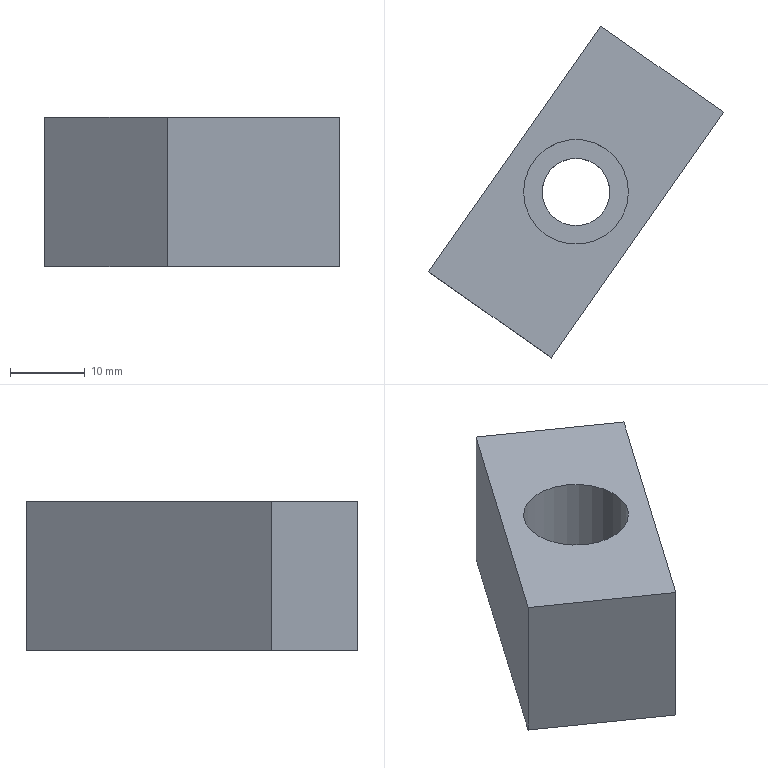Part | NX | features solid 2 | 1 solid | 9 faces | box 39.326 x 44.238 x 20 mm | volume 13824 mm3 | plane 7 | cylinder 2 | commonest cylinder face diameters 9 x1 14 x1
STEP:
#1=CARTESIAN_POINT('',(61.729,209.988,-474.059));
#2=VERTEX_POINT('',#1);
#3=CARTESIAN_POINT('',(66.229,209.988,-474.059));
#4=DIRECTION('',(0.,0.,-1.));
#5=DIRECTION('',(-1.,0.,0.));
#6=AXIS2_PLACEMENT_3D('',#3,#4,#5);
#7=CIRCLE('',#6,4.5);
#8=EDGE_CURVE('',#2,#2,#7,.T.);
#9=ORIENTED_EDGE('',*,*,#8,.F.);
#10=EDGE_LOOP('',(#9));
#11=FACE_BOUND('',#10,.T.);
#12=CARTESIAN_POINT('',(46.566,199.341,-474.059));
#13=VERTEX_POINT('',#12);
#14=CARTESIAN_POINT('',(62.949,187.87,-474.059));
#15=VERTEX_POINT('',#14);
#16=CARTESIAN_POINT('',(79.332,176.398,-474.059));
#17=DIRECTION('',(0.8192,-0.5736,0.));
#18=VECTOR('',#17,1000.);
#19=LINE('',#16,#18);
#20=EDGE_CURVE('',#13,#15,#19,.T.);
#21=ORIENTED_EDGE('',*,*,#20,.F.);
#22=CARTESIAN_POINT('',(69.509,232.107,-474.059));
#23=VERTEX_POINT('',#22);
#24=CARTESIAN_POINT('',(35.381,183.368,-474.059));
#25=DIRECTION('',(0.5736,0.8192,0.));
#26=VECTOR('',#25,1000.);
#27=LINE('',#24,#26);
#28=EDGE_CURVE('',#13,#23,#27,.T.);
#29=ORIENTED_EDGE('',*,*,#28,.T.);
#30=CARTESIAN_POINT('',(85.892,220.636,-474.059));
#31=VERTEX_POINT('',#30);
#32=CARTESIAN_POINT('',(69.509,232.107,-474.059));
#33=DIRECTION('',(0.8192,-0.5736,0.));
#34=VECTOR('',#33,1000.);
#35=LINE('',#32,#34);
#36=EDGE_CURVE('',#23,#31,#35,.T.);
#37=ORIENTED_EDGE('',*,*,#36,.T.);
#38=CARTESIAN_POINT('',(51.765,171.896,-474.059));
#39=DIRECTION('',(0.5736,0.8192,0.));
#40=VECTOR('',#39,1000.);
#41=LINE('',#38,#40);
#42=EDGE_CURVE('',#15,#31,#41,.T.);
#43=ORIENTED_EDGE('',*,*,#42,.F.);
#44=EDGE_LOOP('',(#21,#29,#37,#43));
#45=FACE_BOUND('',#44,.T.);
#46=CARTESIAN_POINT('',(35.381,183.368,-474.059));
#47=DIRECTION('',(0.,0.,-1.));
#48=DIRECTION('',(0.5736,0.8192,0.));
#49=AXIS2_PLACEMENT_3D('',#46,#47,#48);
#50=PLANE('',#49);
#51=ADVANCED_FACE('',(#11,#45),#50,.T.);
#52=ORIENTED_EDGE('',*,*,#36,.F.);
#53=CARTESIAN_POINT('',(69.509,232.107,-454.059));
#54=VERTEX_POINT('',#53);
#55=CARTESIAN_POINT('',(69.509,232.107,-474.059));
#56=DIRECTION('',(0.,0.,1.));
#57=VECTOR('',#56,1000.);
#58=LINE('',#55,#57);
#59=EDGE_CURVE('',#23,#54,#58,.T.);
#60=ORIENTED_EDGE('',*,*,#59,.T.);
#61=CARTESIAN_POINT('',(85.892,220.636,-454.059));
#62=VERTEX_POINT('',#61);
#63=CARTESIAN_POINT('',(69.509,232.107,-454.059));
#64=DIRECTION('',(-0.8192,0.5736,0.));
#65=VECTOR('',#64,1000.);
#66=LINE('',#63,#65);
#67=EDGE_CURVE('',#54,#62,#66,.F.);
#68=ORIENTED_EDGE('',*,*,#67,.T.);
#69=CARTESIAN_POINT('',(85.892,220.636,-474.059));
#70=DIRECTION('',(0.,0.,1.));
#71=VECTOR('',#70,1000.);
#72=LINE('',#69,#71);
#73=EDGE_CURVE('',#31,#62,#72,.T.);
#74=ORIENTED_EDGE('',*,*,#73,.F.);
#75=EDGE_LOOP('',(#52,#60,#68,#74));
#76=FACE_BOUND('',#75,.T.);
#77=CARTESIAN_POINT('',(69.509,232.107,-394.059));
#78=DIRECTION('',(0.5736,0.8192,0.));
#79=DIRECTION('',(0.,0.,1.));
#80=AXIS2_PLACEMENT_3D('',#77,#78,#79);
#81=PLANE('',#80);
#82=ADVANCED_FACE('',(#76),#81,.T.);
#83=CARTESIAN_POINT('',(59.229,209.988,-454.059));
#84=VERTEX_POINT('',#83);
#85=CARTESIAN_POINT('',(66.229,209.988,-454.059));
#86=DIRECTION('',(0.,0.,-1.));
#87=DIRECTION('',(-1.,0.,0.));
#88=AXIS2_PLACEMENT_3D('',#85,#86,#87);
#89=CIRCLE('',#88,7.);
#90=EDGE_CURVE('',#84,#84,#89,.T.);
#91=ORIENTED_EDGE('',*,*,#90,.T.);
#92=EDGE_LOOP('',(#91));
#93=FACE_BOUND('',#92,.T.);
#94=ORIENTED_EDGE('',*,*,#67,.F.);
#95=CARTESIAN_POINT('',(46.566,199.341,-454.059));
#96=VERTEX_POINT('',#95);
#97=CARTESIAN_POINT('',(35.381,183.368,-454.059));
#98=DIRECTION('',(0.5736,0.8192,0.));
#99=VECTOR('',#98,1000.);
#100=LINE('',#97,#99);
#101=EDGE_CURVE('',#96,#54,#100,.T.);
#102=ORIENTED_EDGE('',*,*,#101,.F.);
#103=CARTESIAN_POINT('',(62.949,187.87,-454.059));
#104=VERTEX_POINT('',#103);
#105=CARTESIAN_POINT('',(46.566,199.341,-454.059));
#106=DIRECTION('',(-0.8192,0.5736,0.));
#107=VECTOR('',#106,1000.);
#108=LINE('',#105,#107);
#109=EDGE_CURVE('',#96,#104,#108,.F.);
#110=ORIENTED_EDGE('',*,*,#109,.T.);
#111=CARTESIAN_POINT('',(51.765,171.896,-454.059));
#112=DIRECTION('',(0.5736,0.8192,0.));
#113=VECTOR('',#112,1000.);
#114=LINE('',#111,#113);
#115=EDGE_CURVE('',#104,#62,#114,.T.);
#116=ORIENTED_EDGE('',*,*,#115,.T.);
#117=EDGE_LOOP('',(#94,#102,#110,#116));
#118=FACE_BOUND('',#117,.T.);
#119=CARTESIAN_POINT('',(35.381,183.368,-454.059));
#120=DIRECTION('',(0.,0.,-1.));
#121=DIRECTION('',(0.5736,0.8192,0.));
#122=AXIS2_PLACEMENT_3D('',#119,#120,#121);
#123=PLANE('',#122);
#124=ADVANCED_FACE('',(#93,#118),#123,.F.);
#125=ORIENTED_EDGE('',*,*,#115,.F.);
#126=CARTESIAN_POINT('',(62.949,187.87,-394.059));
#127=DIRECTION('',(0.,0.,1.));
#128=VECTOR('',#127,1000.);
#129=LINE('',#126,#128);
#130=EDGE_CURVE('',#15,#104,#129,.T.);
#131=ORIENTED_EDGE('',*,*,#130,.F.);
#132=ORIENTED_EDGE('',*,*,#42,.T.);
#133=ORIENTED_EDGE('',*,*,#73,.T.);
#134=EDGE_LOOP('',(#125,#131,#132,#133));
#135=FACE_BOUND('',#134,.T.);
#136=CARTESIAN_POINT('',(51.765,171.896,-474.059));
#137=DIRECTION('',(0.8192,-0.5736,0.));
#138=DIRECTION('',(0.5736,0.8192,0.));
#139=AXIS2_PLACEMENT_3D('',#136,#137,#138);
#140=PLANE('',#139);
#141=ADVANCED_FACE('',(#135),#140,.T.);
#142=CARTESIAN_POINT('',(46.566,199.341,-394.059));
#143=DIRECTION('',(0.,0.,1.));
#144=VECTOR('',#143,1000.);
#145=LINE('',#142,#144);
#146=EDGE_CURVE('',#13,#96,#145,.T.);
#147=ORIENTED_EDGE('',*,*,#146,.F.);
#148=ORIENTED_EDGE('',*,*,#20,.T.);
#149=ORIENTED_EDGE('',*,*,#130,.T.);
#150=ORIENTED_EDGE('',*,*,#109,.F.);
#151=EDGE_LOOP('',(#147,#148,#149,#150));
#152=FACE_BOUND('',#151,.T.);
#153=CARTESIAN_POINT('',(79.332,176.398,-394.059));
#154=DIRECTION('',(-0.5736,-0.8192,0.));
#155=DIRECTION('',(0.8192,-0.5736,0.));
#156=AXIS2_PLACEMENT_3D('',#153,#154,#155);
#157=PLANE('',#156);
#158=ADVANCED_FACE('',(#152),#157,.T.);
#159=ORIENTED_EDGE('',*,*,#101,.T.);
#160=ORIENTED_EDGE('',*,*,#59,.F.);
#161=ORIENTED_EDGE('',*,*,#28,.F.);
#162=ORIENTED_EDGE('',*,*,#146,.T.);
#163=EDGE_LOOP('',(#159,#160,#161,#162));
#164=FACE_BOUND('',#163,.T.);
#165=CARTESIAN_POINT('',(35.381,183.368,-474.059));
#166=DIRECTION('',(0.8192,-0.5736,0.));
#167=DIRECTION('',(0.5736,0.8192,0.));
#168=AXIS2_PLACEMENT_3D('',#165,#166,#167);
#169=PLANE('',#168);
#170=ADVANCED_FACE('',(#164),#169,.F.);
#171=ORIENTED_EDGE('',*,*,#8,.T.);
#172=EDGE_LOOP('',(#171));
#173=FACE_BOUND('',#172,.T.);
#174=CARTESIAN_POINT('',(61.729,209.988,-464.059));
#175=VERTEX_POINT('',#174);
#176=CARTESIAN_POINT('',(66.229,209.988,-464.059));
#177=DIRECTION('',(0.,0.,-1.));
#178=DIRECTION('',(-1.,0.,0.));
#179=AXIS2_PLACEMENT_3D('',#176,#177,#178);
#180=CIRCLE('',#179,4.5);
#181=EDGE_CURVE('',#175,#175,#180,.T.);
#182=ORIENTED_EDGE('',*,*,#181,.F.);
#183=EDGE_LOOP('',(#182));
#184=FACE_BOUND('',#183,.T.);
#185=CARTESIAN_POINT('',(66.229,209.988,-504.059));
#186=DIRECTION('',(0.,0.,-1.));
#187=DIRECTION('',(-1.,0.,0.));
#188=AXIS2_PLACEMENT_3D('',#185,#186,#187);
#189=CYLINDRICAL_SURFACE('',#188,4.5);
#190=ADVANCED_FACE('',(#173,#184),#189,.F.);
#191=ORIENTED_EDGE('',*,*,#181,.T.);
#192=EDGE_LOOP('',(#191));
#193=FACE_BOUND('',#192,.T.);
#194=CARTESIAN_POINT('',(59.229,209.988,-464.059));
#195=VERTEX_POINT('',#194);
#196=CARTESIAN_POINT('',(66.229,209.988,-464.059));
#197=DIRECTION('',(0.,0.,-1.));
#198=DIRECTION('',(-1.,0.,0.));
#199=AXIS2_PLACEMENT_3D('',#196,#197,#198);
#200=CIRCLE('',#199,7.);
#201=EDGE_CURVE('',#195,#195,#200,.T.);
#202=ORIENTED_EDGE('',*,*,#201,.F.);
#203=EDGE_LOOP('',(#202));
#204=FACE_BOUND('',#203,.T.);
#205=CARTESIAN_POINT('',(66.229,209.988,-464.059));
#206=DIRECTION('',(0.,0.,-1.));
#207=DIRECTION('',(-1.,0.,0.));
#208=AXIS2_PLACEMENT_3D('',#205,#206,#207);
#209=PLANE('',#208);
#210=ADVANCED_FACE('',(#193,#204),#209,.F.);
#211=ORIENTED_EDGE('',*,*,#201,.T.);
#212=EDGE_LOOP('',(#211));
#213=FACE_BOUND('',#212,.T.);
#214=ORIENTED_EDGE('',*,*,#90,.F.);
#215=EDGE_LOOP('',(#214));
#216=FACE_BOUND('',#215,.T.);
#217=CARTESIAN_POINT('',(66.229,209.988,-454.059));
#218=DIRECTION('',(0.,0.,-1.));
#219=DIRECTION('',(-1.,0.,0.));
#220=AXIS2_PLACEMENT_3D('',#217,#218,#219);
#221=CYLINDRICAL_SURFACE('',#220,7.);
#222=ADVANCED_FACE('',(#213,#216),#221,.F.);
#223=CLOSED_SHELL('',(#51,#82,#124,#141,#158,#170,#190,#210,#222));
#224=MANIFOLD_SOLID_BREP('',#223);
#225=(LENGTH_UNIT()NAMED_UNIT(*)SI_UNIT(.MILLI.,.METRE.));
#226=UNCERTAINTY_MEASURE_WITH_UNIT(LENGTH_MEASURE(0.00001),#225,'','');
#227=(NAMED_UNIT(*)PLANE_ANGLE_UNIT()SI_UNIT($,.RADIAN.));
#228=(NAMED_UNIT(*)SI_UNIT($,.STERADIAN.)SOLID_ANGLE_UNIT());
#229=(GEOMETRIC_REPRESENTATION_CONTEXT(3)GLOBAL_UNCERTAINTY_ASSIGNED_CONTEXT((#226))GLOBAL_UNIT_ASSIGNED_CONTEXT((#225,#227,#228))REPRESENTATION_CONTEXT('',''));
#230=ADVANCED_BREP_SHAPE_REPRESENTATION('',(#224),#229);